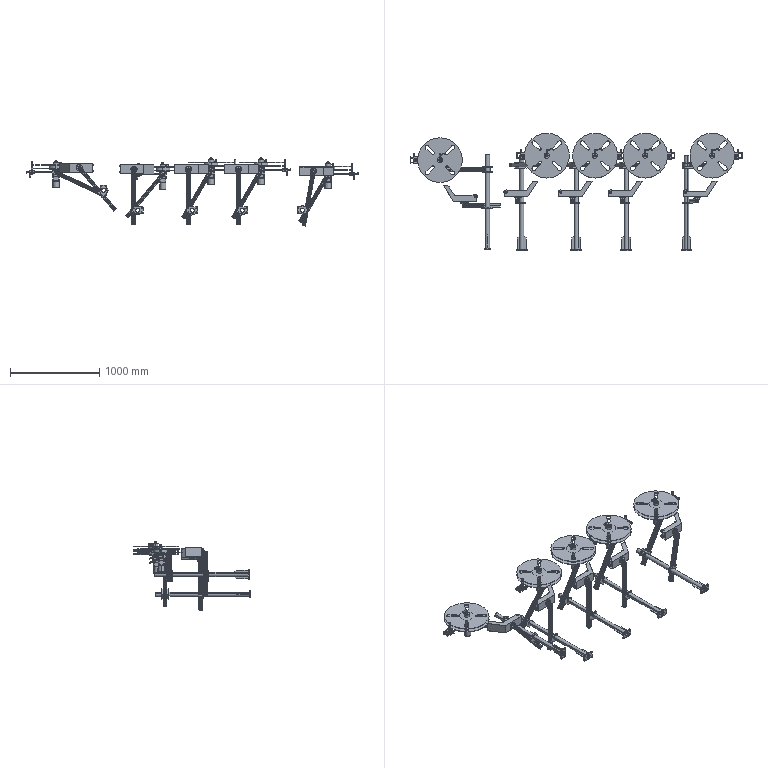Part | NX | 215 solids | 7472 faces | volume 30617630 mm3 | cylinder 2910 | plane 2612 | cone 1465 | torus 285 | spline 150 | sphere 50 | commonest cylinder face diameters 4.2 x220 10 x195 8 x180 6.5 x140 25 x140 19 x130